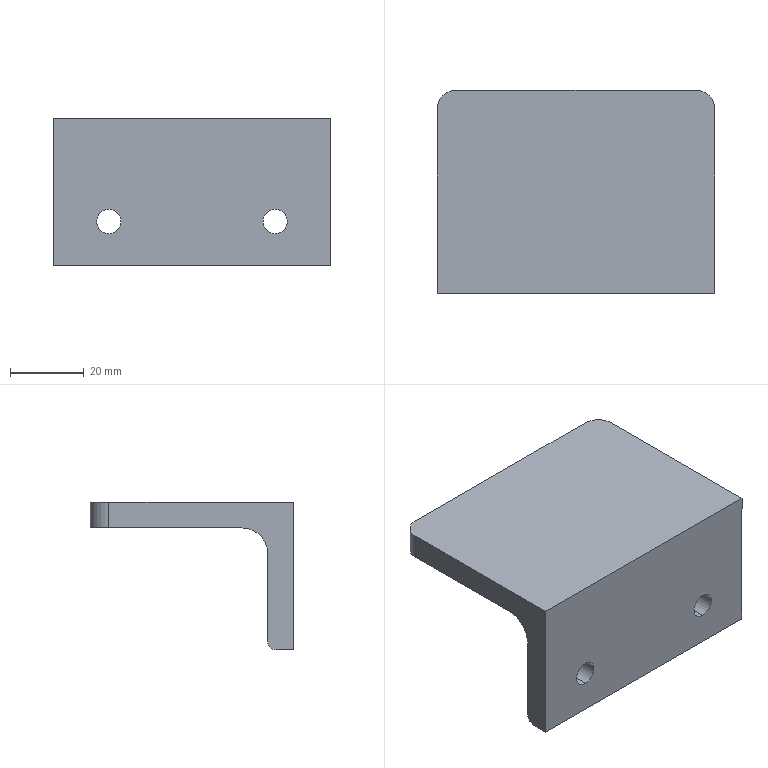Part | SolidWorks | features 3DProfileFeature 1, Fillet 1, HoleWzd 1, ICE 1, WeldMemberFeat 1, WeldmentFeature 1 | 1 solid | 16 faces | box 75 x 55 x 40 mm | volume 46347 mm3 | cylinder 8 | plane 8 | commonest cylinder face diameters 6.6 x4 10 x2 4.667 x1 14 x1
STEP:
#1=CARTESIAN_POINT('',(15.,7.,-24.7));
#2=VERTEX_POINT('',#1);
#3=CARTESIAN_POINT('',(15.,7.,-31.3));
#4=VERTEX_POINT('',#3);
#5=CARTESIAN_POINT('',(15.,7.,-28.));
#6=DIRECTION('',(0.,-1.,0.));
#7=DIRECTION('',(0.,0.,-1.));
#8=AXIS2_PLACEMENT_3D('',#5,#6,#7);
#9=CIRCLE('',#8,3.3);
#10=EDGE_CURVE('',#2,#4,#9,.T.);
#11=ORIENTED_EDGE('',*,*,#10,.F.);
#12=CARTESIAN_POINT('',(15.,0.,-24.7));
#13=VERTEX_POINT('',#12);
#14=CARTESIAN_POINT('',(15.,0.,-24.7));
#15=DIRECTION('',(0.,-1.,0.));
#16=VECTOR('',#15,1000.);
#17=LINE('',#14,#16);
#18=EDGE_CURVE('',#2,#13,#17,.T.);
#19=ORIENTED_EDGE('',*,*,#18,.T.);
#20=CARTESIAN_POINT('',(15.,0.,-31.3));
#21=VERTEX_POINT('',#20);
#22=CARTESIAN_POINT('',(15.,0.,-28.));
#23=DIRECTION('',(0.,-1.,0.));
#24=DIRECTION('',(0.,0.,-1.));
#25=AXIS2_PLACEMENT_3D('',#22,#23,#24);
#26=CIRCLE('',#25,3.3);
#27=EDGE_CURVE('',#13,#21,#26,.T.);
#28=ORIENTED_EDGE('',*,*,#27,.T.);
#29=CARTESIAN_POINT('',(15.,0.,-31.3));
#30=DIRECTION('',(0.,-1.,0.));
#31=VECTOR('',#30,1000.);
#32=LINE('',#29,#31);
#33=EDGE_CURVE('',#4,#21,#32,.T.);
#34=ORIENTED_EDGE('',*,*,#33,.F.);
#35=EDGE_LOOP('',(#11,#19,#28,#34));
#36=FACE_OUTER_BOUND('',#35,.T.);
#37=CARTESIAN_POINT('',(15.,0.,-28.));
#38=DIRECTION('',(0.,-1.,0.));
#39=DIRECTION('',(0.,0.,-1.));
#40=AXIS2_PLACEMENT_3D('',#37,#38,#39);
#41=CYLINDRICAL_SURFACE('',#40,3.3);
#42=ADVANCED_FACE('',(#36),#41,.F.);
#43=CARTESIAN_POINT('',(60.,7.,-24.7));
#44=VERTEX_POINT('',#43);
#45=CARTESIAN_POINT('',(60.,7.,-31.3));
#46=VERTEX_POINT('',#45);
#47=CARTESIAN_POINT('',(60.,7.,-28.));
#48=DIRECTION('',(0.,-1.,0.));
#49=DIRECTION('',(0.,0.,-1.));
#50=AXIS2_PLACEMENT_3D('',#47,#48,#49);
#51=CIRCLE('',#50,3.3);
#52=EDGE_CURVE('',#44,#46,#51,.T.);
#53=ORIENTED_EDGE('',*,*,#52,.F.);
#54=CARTESIAN_POINT('',(60.,0.,-24.7));
#55=VERTEX_POINT('',#54);
#56=CARTESIAN_POINT('',(60.,0.,-24.7));
#57=DIRECTION('',(0.,-1.,0.));
#58=VECTOR('',#57,1000.);
#59=LINE('',#56,#58);
#60=EDGE_CURVE('',#44,#55,#59,.T.);
#61=ORIENTED_EDGE('',*,*,#60,.T.);
#62=CARTESIAN_POINT('',(60.,0.,-31.3));
#63=VERTEX_POINT('',#62);
#64=CARTESIAN_POINT('',(60.,0.,-28.));
#65=DIRECTION('',(0.,-1.,0.));
#66=DIRECTION('',(0.,0.,-1.));
#67=AXIS2_PLACEMENT_3D('',#64,#65,#66);
#68=CIRCLE('',#67,3.3);
#69=EDGE_CURVE('',#55,#63,#68,.T.);
#70=ORIENTED_EDGE('',*,*,#69,.T.);
#71=CARTESIAN_POINT('',(60.,0.,-31.3));
#72=DIRECTION('',(0.,-1.,0.));
#73=VECTOR('',#72,1000.);
#74=LINE('',#71,#73);
#75=EDGE_CURVE('',#46,#63,#74,.T.);
#76=ORIENTED_EDGE('',*,*,#75,.F.);
#77=EDGE_LOOP('',(#53,#61,#70,#76));
#78=FACE_OUTER_BOUND('',#77,.T.);
#79=CARTESIAN_POINT('',(60.,0.,-28.));
#80=DIRECTION('',(0.,-1.,0.));
#81=DIRECTION('',(0.,0.,-1.));
#82=AXIS2_PLACEMENT_3D('',#79,#80,#81);
#83=CYLINDRICAL_SURFACE('',#82,3.3);
#84=ADVANCED_FACE('',(#78),#83,.F.);
#85=CARTESIAN_POINT('',(70.,55.,0.));
#86=VERTEX_POINT('',#85);
#87=CARTESIAN_POINT('',(5.,55.,0.));
#88=VERTEX_POINT('',#87);
#89=CARTESIAN_POINT('',(75.,55.,0.));
#90=DIRECTION('',(-1.,0.,0.));
#91=VECTOR('',#90,1000.);
#92=LINE('',#89,#91);
#93=EDGE_CURVE('',#86,#88,#92,.T.);
#94=ORIENTED_EDGE('',*,*,#93,.T.);
#95=CARTESIAN_POINT('',(0.,50.,0.));
#96=VERTEX_POINT('',#95);
#97=CARTESIAN_POINT('',(5.,50.,0.));
#98=DIRECTION('',(0.,0.,1.));
#99=DIRECTION('',(0.,1.,0.));
#100=AXIS2_PLACEMENT_3D('',#97,#98,#99);
#101=CIRCLE('',#100,5.);
#102=EDGE_CURVE('',#88,#96,#101,.T.);
#103=ORIENTED_EDGE('',*,*,#102,.T.);
#104=CARTESIAN_POINT('',(0.,0.,0.));
#105=VERTEX_POINT('',#104);
#106=CARTESIAN_POINT('',(0.,63.,0.));
#107=DIRECTION('',(0.,-1.,0.));
#108=VECTOR('',#107,1000.);
#109=LINE('',#106,#108);
#110=EDGE_CURVE('',#96,#105,#109,.T.);
#111=ORIENTED_EDGE('',*,*,#110,.T.);
#112=CARTESIAN_POINT('',(75.,0.,0.));
#113=VERTEX_POINT('',#112);
#114=CARTESIAN_POINT('',(75.,0.,0.));
#115=DIRECTION('',(-1.,0.,0.));
#116=VECTOR('',#115,1000.);
#117=LINE('',#114,#116);
#118=EDGE_CURVE('',#113,#105,#117,.T.);
#119=ORIENTED_EDGE('',*,*,#118,.F.);
#120=CARTESIAN_POINT('',(75.,50.,0.));
#121=VERTEX_POINT('',#120);
#122=CARTESIAN_POINT('',(75.,63.,0.));
#123=DIRECTION('',(0.,-1.,0.));
#124=VECTOR('',#123,1000.);
#125=LINE('',#122,#124);
#126=EDGE_CURVE('',#121,#113,#125,.T.);
#127=ORIENTED_EDGE('',*,*,#126,.F.);
#128=CARTESIAN_POINT('',(70.,50.,0.));
#129=DIRECTION('',(0.,0.,1.));
#130=DIRECTION('',(0.,1.,0.));
#131=AXIS2_PLACEMENT_3D('',#128,#129,#130);
#132=CIRCLE('',#131,5.);
#133=EDGE_CURVE('',#121,#86,#132,.T.);
#134=ORIENTED_EDGE('',*,*,#133,.T.);
#135=EDGE_LOOP('',(#94,#103,#111,#119,#127,#134));
#136=FACE_OUTER_BOUND('',#135,.T.);
#137=CARTESIAN_POINT('',(75.,63.,0.));
#138=DIRECTION('',(0.,0.,-1.));
#139=DIRECTION('',(0.,1.,0.));
#140=AXIS2_PLACEMENT_3D('',#137,#138,#139);
#141=PLANE('',#140);
#142=ADVANCED_FACE('',(#136),#141,.F.);
#143=CARTESIAN_POINT('',(15.,0.,-28.));
#144=DIRECTION('',(0.,-1.,0.));
#145=DIRECTION('',(0.,0.,-1.));
#146=AXIS2_PLACEMENT_3D('',#143,#144,#145);
#147=CIRCLE('',#146,3.3);
#148=EDGE_CURVE('',#21,#13,#147,.T.);
#149=ORIENTED_EDGE('',*,*,#148,.F.);
#150=ORIENTED_EDGE('',*,*,#27,.F.);
#151=EDGE_LOOP('',(#149,#150));
#152=FACE_BOUND('',#151,.T.);
#153=CARTESIAN_POINT('',(60.,0.,-28.));
#154=DIRECTION('',(0.,-1.,0.));
#155=DIRECTION('',(0.,0.,-1.));
#156=AXIS2_PLACEMENT_3D('',#153,#154,#155);
#157=CIRCLE('',#156,3.3);
#158=EDGE_CURVE('',#63,#55,#157,.T.);
#159=ORIENTED_EDGE('',*,*,#158,.F.);
#160=ORIENTED_EDGE('',*,*,#69,.F.);
#161=EDGE_LOOP('',(#159,#160));
#162=FACE_BOUND('',#161,.T.);
#163=CARTESIAN_POINT('',(0.,0.,-40.));
#164=VERTEX_POINT('',#163);
#165=CARTESIAN_POINT('',(0.,0.,0.));
#166=DIRECTION('',(0.,0.,-1.));
#167=VECTOR('',#166,1000.);
#168=LINE('',#165,#167);
#169=EDGE_CURVE('',#105,#164,#168,.T.);
#170=ORIENTED_EDGE('',*,*,#169,.T.);
#171=CARTESIAN_POINT('',(75.,0.,-40.));
#172=VERTEX_POINT('',#171);
#173=CARTESIAN_POINT('',(75.,0.,-40.));
#174=DIRECTION('',(-1.,0.,0.));
#175=VECTOR('',#174,1000.);
#176=LINE('',#173,#175);
#177=EDGE_CURVE('',#172,#164,#176,.T.);
#178=ORIENTED_EDGE('',*,*,#177,.F.);
#179=CARTESIAN_POINT('',(75.,0.,0.));
#180=DIRECTION('',(0.,0.,-1.));
#181=VECTOR('',#180,1000.);
#182=LINE('',#179,#181);
#183=EDGE_CURVE('',#113,#172,#182,.T.);
#184=ORIENTED_EDGE('',*,*,#183,.F.);
#185=ORIENTED_EDGE('',*,*,#118,.T.);
#186=EDGE_LOOP('',(#170,#178,#184,#185));
#187=FACE_OUTER_BOUND('',#186,.T.);
#188=CARTESIAN_POINT('',(75.,0.,0.));
#189=DIRECTION('',(0.,1.,0.));
#190=DIRECTION('',(0.,0.,1.));
#191=AXIS2_PLACEMENT_3D('',#188,#189,#190);
#192=PLANE('',#191);
#193=ADVANCED_FACE('',(#152,#162,#187),#192,.F.);
#194=CARTESIAN_POINT('',(0.,4.667,-40.));
#195=VERTEX_POINT('',#194);
#196=CARTESIAN_POINT('',(0.,0.,-40.));
#197=DIRECTION('',(0.,1.,0.));
#198=VECTOR('',#197,1000.);
#199=LINE('',#196,#198);
#200=EDGE_CURVE('',#164,#195,#199,.T.);
#201=ORIENTED_EDGE('',*,*,#200,.T.);
#202=CARTESIAN_POINT('',(75.,4.667,-40.));
#203=VERTEX_POINT('',#202);
#204=CARTESIAN_POINT('',(75.,4.667,-40.));
#205=DIRECTION('',(-1.,0.,0.));
#206=VECTOR('',#205,1000.);
#207=LINE('',#204,#206);
#208=EDGE_CURVE('',#203,#195,#207,.T.);
#209=ORIENTED_EDGE('',*,*,#208,.F.);
#210=CARTESIAN_POINT('',(75.,0.,-40.));
#211=DIRECTION('',(0.,1.,0.));
#212=VECTOR('',#211,1000.);
#213=LINE('',#210,#212);
#214=EDGE_CURVE('',#172,#203,#213,.T.);
#215=ORIENTED_EDGE('',*,*,#214,.F.);
#216=ORIENTED_EDGE('',*,*,#177,.T.);
#217=EDGE_LOOP('',(#201,#209,#215,#216));
#218=FACE_OUTER_BOUND('',#217,.T.);
#219=CARTESIAN_POINT('',(75.,0.,-40.));
#220=DIRECTION('',(0.,0.,1.));
#221=DIRECTION('',(0.,-1.,0.));
#222=AXIS2_PLACEMENT_3D('',#219,#220,#221);
#223=PLANE('',#222);
#224=ADVANCED_FACE('',(#218),#223,.F.);
#225=CARTESIAN_POINT('',(0.,7.,-37.667));
#226=VERTEX_POINT('',#225);
#227=CARTESIAN_POINT('',(0.,4.667,-37.667));
#228=DIRECTION('',(1.,0.,0.));
#229=DIRECTION('',(0.,0.,-1.));
#230=AXIS2_PLACEMENT_3D('',#227,#228,#229);
#231=CIRCLE('',#230,2.333);
#232=EDGE_CURVE('',#195,#226,#231,.T.);
#233=ORIENTED_EDGE('',*,*,#232,.T.);
#234=CARTESIAN_POINT('',(75.,7.,-37.667));
#235=VERTEX_POINT('',#234);
#236=CARTESIAN_POINT('',(75.,7.,-37.667));
#237=DIRECTION('',(-1.,0.,0.));
#238=VECTOR('',#237,1000.);
#239=LINE('',#236,#238);
#240=EDGE_CURVE('',#235,#226,#239,.T.);
#241=ORIENTED_EDGE('',*,*,#240,.F.);
#242=CARTESIAN_POINT('',(75.,4.667,-37.667));
#243=DIRECTION('',(1.,0.,0.));
#244=DIRECTION('',(0.,0.,-1.));
#245=AXIS2_PLACEMENT_3D('',#242,#243,#244);
#246=CIRCLE('',#245,2.333);
#247=EDGE_CURVE('',#203,#235,#246,.T.);
#248=ORIENTED_EDGE('',*,*,#247,.F.);
#249=ORIENTED_EDGE('',*,*,#208,.T.);
#250=EDGE_LOOP('',(#233,#241,#248,#249));
#251=FACE_OUTER_BOUND('',#250,.T.);
#252=CARTESIAN_POINT('',(75.,4.667,-37.667));
#253=DIRECTION('',(-1.,0.,0.));
#254=DIRECTION('',(0.,0.,1.));
#255=AXIS2_PLACEMENT_3D('',#252,#253,#254);
#256=CYLINDRICAL_SURFACE('',#255,2.333);
#257=ADVANCED_FACE('',(#251),#256,.T.);
#258=CARTESIAN_POINT('',(15.,7.,-28.));
#259=DIRECTION('',(0.,-1.,0.));
#260=DIRECTION('',(0.,0.,-1.));
#261=AXIS2_PLACEMENT_3D('',#258,#259,#260);
#262=CIRCLE('',#261,3.3);
#263=EDGE_CURVE('',#4,#2,#262,.T.);
#264=ORIENTED_EDGE('',*,*,#263,.T.);
#265=ORIENTED_EDGE('',*,*,#10,.T.);
#266=EDGE_LOOP('',(#264,#265));
#267=FACE_BOUND('',#266,.T.);
#268=CARTESIAN_POINT('',(60.,7.,-28.));
#269=DIRECTION('',(0.,-1.,0.));
#270=DIRECTION('',(0.,0.,-1.));
#271=AXIS2_PLACEMENT_3D('',#268,#269,#270);
#272=CIRCLE('',#271,3.3);
#273=EDGE_CURVE('',#46,#44,#272,.T.);
#274=ORIENTED_EDGE('',*,*,#273,.T.);
#275=ORIENTED_EDGE('',*,*,#52,.T.);
#276=EDGE_LOOP('',(#274,#275));
#277=FACE_BOUND('',#276,.T.);
#278=CARTESIAN_POINT('',(0.,7.,-14.));
#279=VERTEX_POINT('',#278);
#280=CARTESIAN_POINT('',(0.,7.,-14.));
#281=DIRECTION('',(0.,0.,1.));
#282=VECTOR('',#281,1000.);
#283=LINE('',#280,#282);
#284=EDGE_CURVE('',#226,#279,#283,.T.);
#285=ORIENTED_EDGE('',*,*,#284,.T.);
#286=CARTESIAN_POINT('',(75.,7.,-14.));
#287=VERTEX_POINT('',#286);
#288=CARTESIAN_POINT('',(75.,7.,-14.));
#289=DIRECTION('',(-1.,0.,0.));
#290=VECTOR('',#289,1000.);
#291=LINE('',#288,#290);
#292=EDGE_CURVE('',#287,#279,#291,.T.);
#293=ORIENTED_EDGE('',*,*,#292,.F.);
#294=CARTESIAN_POINT('',(75.,7.,-14.));
#295=DIRECTION('',(0.,0.,1.));
#296=VECTOR('',#295,1000.);
#297=LINE('',#294,#296);
#298=EDGE_CURVE('',#235,#287,#297,.T.);
#299=ORIENTED_EDGE('',*,*,#298,.F.);
#300=ORIENTED_EDGE('',*,*,#240,.T.);
#301=EDGE_LOOP('',(#285,#293,#299,#300));
#302=FACE_OUTER_BOUND('',#301,.T.);
#303=CARTESIAN_POINT('',(75.,7.,-14.));
#304=DIRECTION('',(0.,-1.,0.));
#305=DIRECTION('',(0.,0.,-1.));
#306=AXIS2_PLACEMENT_3D('',#303,#304,#305);
#307=PLANE('',#306);
#308=ADVANCED_FACE('',(#267,#277,#302),#307,.F.);
#309=CARTESIAN_POINT('',(0.,14.,-7.));
#310=VERTEX_POINT('',#309);
#311=CARTESIAN_POINT('',(0.,14.,-14.));
#312=DIRECTION('',(-1.,0.,0.));
#313=DIRECTION('',(0.,0.,-1.));
#314=AXIS2_PLACEMENT_3D('',#311,#312,#313);
#315=CIRCLE('',#314,7.);
#316=EDGE_CURVE('',#279,#310,#315,.T.);
#317=ORIENTED_EDGE('',*,*,#316,.T.);
#318=CARTESIAN_POINT('',(75.,14.,-7.));
#319=VERTEX_POINT('',#318);
#320=CARTESIAN_POINT('',(75.,14.,-7.));
#321=DIRECTION('',(-1.,0.,0.));
#322=VECTOR('',#321,1000.);
#323=LINE('',#320,#322);
#324=EDGE_CURVE('',#319,#310,#323,.T.);
#325=ORIENTED_EDGE('',*,*,#324,.F.);
#326=CARTESIAN_POINT('',(75.,14.,-14.));
#327=DIRECTION('',(-1.,0.,0.));
#328=DIRECTION('',(0.,0.,-1.));
#329=AXIS2_PLACEMENT_3D('',#326,#327,#328);
#330=CIRCLE('',#329,7.);
#331=EDGE_CURVE('',#287,#319,#330,.T.);
#332=ORIENTED_EDGE('',*,*,#331,.F.);
#333=ORIENTED_EDGE('',*,*,#292,.T.);
#334=EDGE_LOOP('',(#317,#325,#332,#333));
#335=FACE_OUTER_BOUND('',#334,.T.);
#336=CARTESIAN_POINT('',(75.,14.,-14.));
#337=DIRECTION('',(-1.,0.,0.));
#338=DIRECTION('',(0.,0.,1.));
#339=AXIS2_PLACEMENT_3D('',#336,#337,#338);
#340=CYLINDRICAL_SURFACE('',#339,7.);
#341=ADVANCED_FACE('',(#335),#340,.F.);
#342=CARTESIAN_POINT('',(0.,50.,-7.));
#343=VERTEX_POINT('',#342);
#344=CARTESIAN_POINT('',(0.,60.667,-7.));
#345=DIRECTION('',(0.,1.,0.));
#346=VECTOR('',#345,1000.);
#347=LINE('',#344,#346);
#348=EDGE_CURVE('',#310,#343,#347,.T.);
#349=ORIENTED_EDGE('',*,*,#348,.T.);
#350=CARTESIAN_POINT('',(5.,55.,-7.));
#351=VERTEX_POINT('',#350);
#352=CARTESIAN_POINT('',(5.,50.,-7.));
#353=DIRECTION('',(0.,0.,-1.));
#354=DIRECTION('',(0.,-1.,0.));
#355=AXIS2_PLACEMENT_3D('',#352,#353,#354);
#356=CIRCLE('',#355,5.);
#357=EDGE_CURVE('',#343,#351,#356,.T.);
#358=ORIENTED_EDGE('',*,*,#357,.T.);
#359=CARTESIAN_POINT('',(70.,55.,-7.));
#360=VERTEX_POINT('',#359);
#361=CARTESIAN_POINT('',(0.,55.,-7.));
#362=DIRECTION('',(1.,0.,0.));
#363=VECTOR('',#362,1000.);
#364=LINE('',#361,#363);
#365=EDGE_CURVE('',#351,#360,#364,.T.);
#366=ORIENTED_EDGE('',*,*,#365,.T.);
#367=CARTESIAN_POINT('',(75.,50.,-7.));
#368=VERTEX_POINT('',#367);
#369=CARTESIAN_POINT('',(70.,50.,-7.));
#370=DIRECTION('',(0.,0.,-1.));
#371=DIRECTION('',(0.,-1.,0.));
#372=AXIS2_PLACEMENT_3D('',#369,#370,#371);
#373=CIRCLE('',#372,5.);
#374=EDGE_CURVE('',#360,#368,#373,.T.);
#375=ORIENTED_EDGE('',*,*,#374,.T.);
#376=CARTESIAN_POINT('',(75.,60.667,-7.));
#377=DIRECTION('',(0.,1.,0.));
#378=VECTOR('',#377,1000.);
#379=LINE('',#376,#378);
#380=EDGE_CURVE('',#319,#368,#379,.T.);
#381=ORIENTED_EDGE('',*,*,#380,.F.);
#382=ORIENTED_EDGE('',*,*,#324,.T.);
#383=EDGE_LOOP('',(#349,#358,#366,#375,#381,#382));
#384=FACE_OUTER_BOUND('',#383,.T.);
#385=CARTESIAN_POINT('',(75.,60.667,-7.));
#386=DIRECTION('',(0.,0.,1.));
#387=DIRECTION('',(0.,-1.,0.));
#388=AXIS2_PLACEMENT_3D('',#385,#386,#387);
#389=PLANE('',#388);
#390=ADVANCED_FACE('',(#384),#389,.F.);
#391=ORIENTED_EDGE('',*,*,#380,.T.);
#392=CARTESIAN_POINT('',(75.,50.,-4.667));
#393=DIRECTION('',(0.,0.,1.));
#394=VECTOR('',#393,1000.);
#395=LINE('',#392,#394);
#396=EDGE_CURVE('',#368,#121,#395,.T.);
#397=ORIENTED_EDGE('',*,*,#396,.T.);
#398=ORIENTED_EDGE('',*,*,#126,.T.);
#399=ORIENTED_EDGE('',*,*,#183,.T.);
#400=ORIENTED_EDGE('',*,*,#214,.T.);
#401=ORIENTED_EDGE('',*,*,#247,.T.);
#402=ORIENTED_EDGE('',*,*,#298,.T.);
#403=ORIENTED_EDGE('',*,*,#331,.T.);
#404=EDGE_LOOP('',(#391,#397,#398,#399,#400,#401,#402,#403));
#405=FACE_OUTER_BOUND('',#404,.T.);
#406=CARTESIAN_POINT('',(75.,60.667,-4.667));
#407=DIRECTION('',(-1.,0.,0.));
#408=DIRECTION('',(0.,0.,1.));
#409=AXIS2_PLACEMENT_3D('',#406,#407,#408);
#410=PLANE('',#409);
#411=ADVANCED_FACE('',(#405),#410,.F.);
#412=ORIENTED_EDGE('',*,*,#110,.F.);
#413=CARTESIAN_POINT('',(0.,50.,-7.));
#414=DIRECTION('',(0.,0.,-1.));
#415=VECTOR('',#414,1000.);
#416=LINE('',#413,#415);
#417=EDGE_CURVE('',#96,#343,#416,.T.);
#418=ORIENTED_EDGE('',*,*,#417,.T.);
#419=ORIENTED_EDGE('',*,*,#348,.F.);
#420=ORIENTED_EDGE('',*,*,#316,.F.);
#421=ORIENTED_EDGE('',*,*,#284,.F.);
#422=ORIENTED_EDGE('',*,*,#232,.F.);
#423=ORIENTED_EDGE('',*,*,#200,.F.);
#424=ORIENTED_EDGE('',*,*,#169,.F.);
#425=EDGE_LOOP('',(#412,#418,#419,#420,#421,#422,#423,#424));
#426=FACE_OUTER_BOUND('',#425,.T.);
#427=CARTESIAN_POINT('',(0.,60.667,-4.667));
#428=DIRECTION('',(-1.,0.,0.));
#429=DIRECTION('',(0.,0.,1.));
#430=AXIS2_PLACEMENT_3D('',#427,#428,#429);
#431=PLANE('',#430);
#432=ADVANCED_FACE('',(#426),#431,.T.);
#433=ORIENTED_EDGE('',*,*,#60,.F.);
#434=ORIENTED_EDGE('',*,*,#273,.F.);
#435=ORIENTED_EDGE('',*,*,#75,.T.);
#436=ORIENTED_EDGE('',*,*,#158,.T.);
#437=EDGE_LOOP('',(#433,#434,#435,#436));
#438=FACE_OUTER_BOUND('',#437,.T.);
#439=CARTESIAN_POINT('',(60.,0.,-28.));
#440=DIRECTION('',(0.,-1.,0.));
#441=DIRECTION('',(0.,0.,-1.));
#442=AXIS2_PLACEMENT_3D('',#439,#440,#441);
#443=CYLINDRICAL_SURFACE('',#442,3.3);
#444=ADVANCED_FACE('',(#438),#443,.F.);
#445=ORIENTED_EDGE('',*,*,#18,.F.);
#446=ORIENTED_EDGE('',*,*,#263,.F.);
#447=ORIENTED_EDGE('',*,*,#33,.T.);
#448=ORIENTED_EDGE('',*,*,#148,.T.);
#449=EDGE_LOOP('',(#445,#446,#447,#448));
#450=FACE_OUTER_BOUND('',#449,.T.);
#451=CARTESIAN_POINT('',(15.,0.,-28.));
#452=DIRECTION('',(0.,-1.,0.));
#453=DIRECTION('',(0.,0.,-1.));
#454=AXIS2_PLACEMENT_3D('',#451,#452,#453);
#455=CYLINDRICAL_SURFACE('',#454,3.3);
#456=ADVANCED_FACE('',(#450),#455,.F.);
#457=ORIENTED_EDGE('',*,*,#365,.F.);
#458=CARTESIAN_POINT('',(5.,55.,0.));
#459=DIRECTION('',(0.,0.,1.));
#460=VECTOR('',#459,1000.);
#461=LINE('',#458,#460);
#462=EDGE_CURVE('',#351,#88,#461,.T.);
#463=ORIENTED_EDGE('',*,*,#462,.T.);
#464=ORIENTED_EDGE('',*,*,#93,.F.);
#465=CARTESIAN_POINT('',(70.,55.,7.));
#466=DIRECTION('',(0.,0.,-1.));
#467=VECTOR('',#466,1000.);
#468=LINE('',#465,#467);
#469=EDGE_CURVE('',#86,#360,#468,.T.);
#470=ORIENTED_EDGE('',*,*,#469,.T.);
#471=EDGE_LOOP('',(#457,#463,#464,#470));
#472=FACE_OUTER_BOUND('',#471,.T.);
#473=CARTESIAN_POINT('',(0.,55.,7.));
#474=DIRECTION('',(0.,-1.,0.));
#475=DIRECTION('',(0.,0.,-1.));
#476=AXIS2_PLACEMENT_3D('',#473,#474,#475);
#477=PLANE('',#476);
#478=ADVANCED_FACE('',(#472),#477,.F.);
#479=ORIENTED_EDGE('',*,*,#357,.F.);
#480=ORIENTED_EDGE('',*,*,#417,.F.);
#481=ORIENTED_EDGE('',*,*,#102,.F.);
#482=ORIENTED_EDGE('',*,*,#462,.F.);
#483=EDGE_LOOP('',(#479,#480,#481,#482));
#484=FACE_OUTER_BOUND('',#483,.T.);
#485=CARTESIAN_POINT('',(5.,50.,7.));
#486=DIRECTION('',(0.,0.,-1.));
#487=DIRECTION('',(-1.,0.,0.));
#488=AXIS2_PLACEMENT_3D('',#485,#486,#487);
#489=CYLINDRICAL_SURFACE('',#488,5.);
#490=ADVANCED_FACE('',(#484),#489,.T.);
#491=ORIENTED_EDGE('',*,*,#374,.F.);
#492=ORIENTED_EDGE('',*,*,#469,.F.);
#493=ORIENTED_EDGE('',*,*,#133,.F.);
#494=ORIENTED_EDGE('',*,*,#396,.F.);
#495=EDGE_LOOP('',(#491,#492,#493,#494));
#496=FACE_OUTER_BOUND('',#495,.T.);
#497=CARTESIAN_POINT('',(70.,50.,-4.667));
#498=DIRECTION('',(0.,0.,1.));
#499=DIRECTION('',(1.,0.,0.));
#500=AXIS2_PLACEMENT_3D('',#497,#498,#499);
#501=CYLINDRICAL_SURFACE('',#500,5.);
#502=ADVANCED_FACE('',(#496),#501,.T.);
#503=CLOSED_SHELL('',(#42,#84,#142,#193,#224,#257,#308,#341,#390,#411,#432,#444,#456,#478,#490,#502));
#504=MANIFOLD_SOLID_BREP('',#503);
#505=CARTESIAN_POINT('',(0.,0.,0.));
#506=DIRECTION('',(0.,0.,1.));
#507=DIRECTION('',(1.,0.,0.));
#508=AXIS2_PLACEMENT_3D('',#505,#506,#507);
#509=(LENGTH_UNIT()NAMED_UNIT(*)SI_UNIT(.MILLI.,.METRE.));
#510=UNCERTAINTY_MEASURE_WITH_UNIT(LENGTH_MEASURE(0.00001),#509,'','');
#511=(NAMED_UNIT(*)PLANE_ANGLE_UNIT()SI_UNIT($,.RADIAN.));
#512=(NAMED_UNIT(*)SI_UNIT($,.STERADIAN.)SOLID_ANGLE_UNIT());
#513=(GEOMETRIC_REPRESENTATION_CONTEXT(3)GLOBAL_UNCERTAINTY_ASSIGNED_CONTEXT((#510))GLOBAL_UNIT_ASSIGNED_CONTEXT((#509,#511,#512))REPRESENTATION_CONTEXT('',''));
#514=ADVANCED_BREP_SHAPE_REPRESENTATION('',(#504,#508),#513);